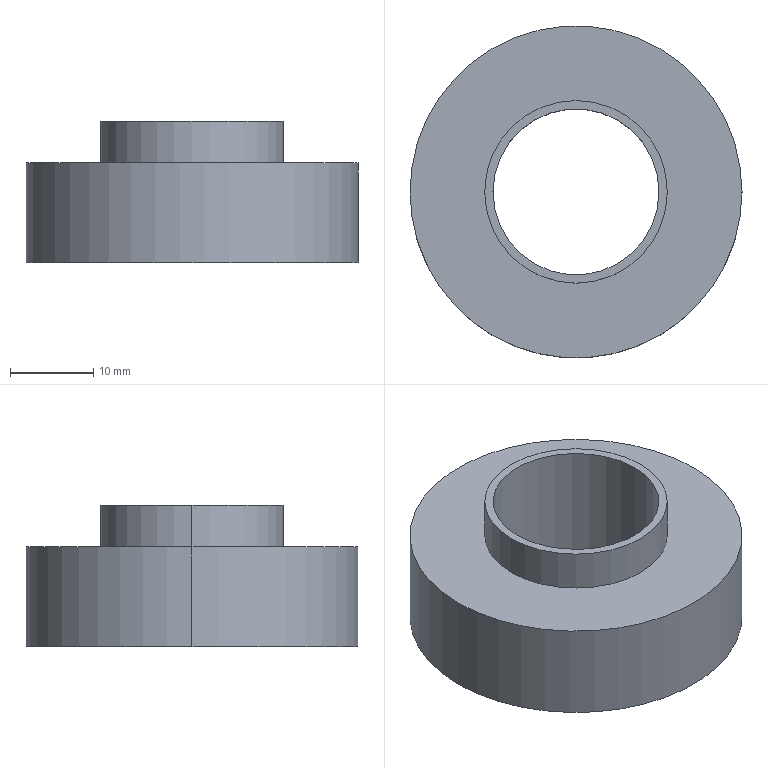Part | SolidWorks | features Extrusion 1, ICE 1 | 1 solid | 9 faces | box 40 x 40 x 17 mm | volume 11640 mm3 | cylinder 6 | plane 3 | commonest cylinder face diameters 20 x2 22 x2 40 x2
STEP:
#1=CARTESIAN_POINT('',(11.,0.,17.));
#2=VERTEX_POINT('',#1);
#3=CARTESIAN_POINT('',(-11.,0.,17.));
#4=VERTEX_POINT('',#3);
#5=CARTESIAN_POINT('',(0.,0.,17.));
#6=DIRECTION('',(0.,0.,1.));
#7=DIRECTION('',(1.,0.,0.));
#8=AXIS2_PLACEMENT_3D('',#5,#6,#7);
#9=CIRCLE('',#8,11.);
#10=EDGE_CURVE('',#2,#4,#9,.T.);
#11=ORIENTED_EDGE('',*,*,#10,.F.);
#12=CARTESIAN_POINT('',(11.,0.,12.));
#13=VERTEX_POINT('',#12);
#14=CARTESIAN_POINT('',(11.,0.,17.));
#15=DIRECTION('',(0.,0.,-1.));
#16=VECTOR('',#15,1000.);
#17=LINE('',#14,#16);
#18=EDGE_CURVE('',#2,#13,#17,.T.);
#19=ORIENTED_EDGE('',*,*,#18,.T.);
#20=CARTESIAN_POINT('',(-11.,0.,12.));
#21=VERTEX_POINT('',#20);
#22=CARTESIAN_POINT('',(0.,0.,12.));
#23=DIRECTION('',(0.,0.,1.));
#24=DIRECTION('',(1.,0.,0.));
#25=AXIS2_PLACEMENT_3D('',#22,#23,#24);
#26=CIRCLE('',#25,11.);
#27=EDGE_CURVE('',#13,#21,#26,.T.);
#28=ORIENTED_EDGE('',*,*,#27,.T.);
#29=CARTESIAN_POINT('',(-11.,0.,17.));
#30=DIRECTION('',(0.,0.,-1.));
#31=VECTOR('',#30,1000.);
#32=LINE('',#29,#31);
#33=EDGE_CURVE('',#4,#21,#32,.T.);
#34=ORIENTED_EDGE('',*,*,#33,.F.);
#35=EDGE_LOOP('',(#11,#19,#28,#34));
#36=FACE_OUTER_BOUND('',#35,.T.);
#37=CARTESIAN_POINT('',(0.,0.,17.));
#38=DIRECTION('',(0.,0.,-1.));
#39=DIRECTION('',(-1.,0.,0.));
#40=AXIS2_PLACEMENT_3D('',#37,#38,#39);
#41=CYLINDRICAL_SURFACE('',#40,11.);
#42=ADVANCED_FACE('',(#36),#41,.T.);
#43=CARTESIAN_POINT('',(-10.,0.,17.));
#44=VERTEX_POINT('',#43);
#45=CARTESIAN_POINT('',(10.,0.,17.));
#46=VERTEX_POINT('',#45);
#47=CARTESIAN_POINT('',(0.,0.,17.));
#48=DIRECTION('',(0.,0.,1.));
#49=DIRECTION('',(1.,0.,0.));
#50=AXIS2_PLACEMENT_3D('',#47,#48,#49);
#51=CIRCLE('',#50,10.);
#52=EDGE_CURVE('',#44,#46,#51,.T.);
#53=ORIENTED_EDGE('',*,*,#52,.T.);
#54=CARTESIAN_POINT('',(10.,0.,0.));
#55=VERTEX_POINT('',#54);
#56=CARTESIAN_POINT('',(10.,0.,12.));
#57=DIRECTION('',(0.,0.,-1.));
#58=VECTOR('',#57,1000.);
#59=LINE('',#56,#58);
#60=EDGE_CURVE('',#46,#55,#59,.T.);
#61=ORIENTED_EDGE('',*,*,#60,.T.);
#62=CARTESIAN_POINT('',(-10.,0.,0.));
#63=VERTEX_POINT('',#62);
#64=CARTESIAN_POINT('',(0.,0.,0.));
#65=DIRECTION('',(0.,0.,1.));
#66=DIRECTION('',(1.,0.,0.));
#67=AXIS2_PLACEMENT_3D('',#64,#65,#66);
#68=CIRCLE('',#67,10.);
#69=EDGE_CURVE('',#63,#55,#68,.T.);
#70=ORIENTED_EDGE('',*,*,#69,.F.);
#71=CARTESIAN_POINT('',(-10.,0.,12.));
#72=DIRECTION('',(0.,0.,-1.));
#73=VECTOR('',#72,1000.);
#74=LINE('',#71,#73);
#75=EDGE_CURVE('',#44,#63,#74,.T.);
#76=ORIENTED_EDGE('',*,*,#75,.F.);
#77=EDGE_LOOP('',(#53,#61,#70,#76));
#78=FACE_OUTER_BOUND('',#77,.T.);
#79=CARTESIAN_POINT('',(0.,0.,12.));
#80=DIRECTION('',(0.,0.,-1.));
#81=DIRECTION('',(-1.,0.,0.));
#82=AXIS2_PLACEMENT_3D('',#79,#80,#81);
#83=CYLINDRICAL_SURFACE('',#82,10.);
#84=ADVANCED_FACE('',(#78),#83,.F.);
#85=CARTESIAN_POINT('',(20.,0.,12.));
#86=VERTEX_POINT('',#85);
#87=CARTESIAN_POINT('',(-20.,0.,12.));
#88=VERTEX_POINT('',#87);
#89=CARTESIAN_POINT('',(0.,0.,12.));
#90=DIRECTION('',(0.,0.,1.));
#91=DIRECTION('',(1.,0.,0.));
#92=AXIS2_PLACEMENT_3D('',#89,#90,#91);
#93=CIRCLE('',#92,20.);
#94=EDGE_CURVE('',#86,#88,#93,.T.);
#95=ORIENTED_EDGE('',*,*,#94,.F.);
#96=CARTESIAN_POINT('',(20.,0.,0.));
#97=VERTEX_POINT('',#96);
#98=CARTESIAN_POINT('',(20.,0.,12.));
#99=DIRECTION('',(0.,0.,-1.));
#100=VECTOR('',#99,1000.);
#101=LINE('',#98,#100);
#102=EDGE_CURVE('',#86,#97,#101,.T.);
#103=ORIENTED_EDGE('',*,*,#102,.T.);
#104=CARTESIAN_POINT('',(-20.,0.,0.));
#105=VERTEX_POINT('',#104);
#106=CARTESIAN_POINT('',(0.,0.,0.));
#107=DIRECTION('',(0.,0.,1.));
#108=DIRECTION('',(1.,0.,0.));
#109=AXIS2_PLACEMENT_3D('',#106,#107,#108);
#110=CIRCLE('',#109,20.);
#111=EDGE_CURVE('',#97,#105,#110,.T.);
#112=ORIENTED_EDGE('',*,*,#111,.T.);
#113=CARTESIAN_POINT('',(-20.,0.,12.));
#114=DIRECTION('',(0.,0.,-1.));
#115=VECTOR('',#114,1000.);
#116=LINE('',#113,#115);
#117=EDGE_CURVE('',#88,#105,#116,.T.);
#118=ORIENTED_EDGE('',*,*,#117,.F.);
#119=EDGE_LOOP('',(#95,#103,#112,#118));
#120=FACE_OUTER_BOUND('',#119,.T.);
#121=CARTESIAN_POINT('',(0.,0.,12.));
#122=DIRECTION('',(0.,0.,-1.));
#123=DIRECTION('',(-1.,0.,0.));
#124=AXIS2_PLACEMENT_3D('',#121,#122,#123);
#125=CYLINDRICAL_SURFACE('',#124,20.);
#126=ADVANCED_FACE('',(#120),#125,.T.);
#127=CARTESIAN_POINT('',(0.,0.,12.));
#128=DIRECTION('',(0.,0.,1.));
#129=DIRECTION('',(1.,0.,0.));
#130=AXIS2_PLACEMENT_3D('',#127,#128,#129);
#131=CIRCLE('',#130,20.);
#132=EDGE_CURVE('',#88,#86,#131,.T.);
#133=ORIENTED_EDGE('',*,*,#132,.T.);
#134=ORIENTED_EDGE('',*,*,#94,.T.);
#135=EDGE_LOOP('',(#133,#134));
#136=FACE_OUTER_BOUND('',#135,.T.);
#137=CARTESIAN_POINT('',(0.,0.,12.));
#138=DIRECTION('',(0.,0.,1.));
#139=DIRECTION('',(1.,0.,0.));
#140=AXIS2_PLACEMENT_3D('',#137,#138,#139);
#141=CIRCLE('',#140,11.);
#142=EDGE_CURVE('',#21,#13,#141,.T.);
#143=ORIENTED_EDGE('',*,*,#142,.F.);
#144=ORIENTED_EDGE('',*,*,#27,.F.);
#145=EDGE_LOOP('',(#143,#144));
#146=FACE_BOUND('',#145,.T.);
#147=CARTESIAN_POINT('',(0.,0.,12.));
#148=DIRECTION('',(0.,0.,1.));
#149=DIRECTION('',(1.,0.,0.));
#150=AXIS2_PLACEMENT_3D('',#147,#148,#149);
#151=PLANE('',#150);
#152=ADVANCED_FACE('',(#136,#146),#151,.T.);
#153=CARTESIAN_POINT('',(0.,0.,0.));
#154=DIRECTION('',(0.,0.,1.));
#155=DIRECTION('',(1.,0.,0.));
#156=AXIS2_PLACEMENT_3D('',#153,#154,#155);
#157=CIRCLE('',#156,20.);
#158=EDGE_CURVE('',#105,#97,#157,.T.);
#159=ORIENTED_EDGE('',*,*,#158,.F.);
#160=ORIENTED_EDGE('',*,*,#111,.F.);
#161=EDGE_LOOP('',(#159,#160));
#162=FACE_OUTER_BOUND('',#161,.T.);
#163=ORIENTED_EDGE('',*,*,#69,.T.);
#164=CARTESIAN_POINT('',(0.,0.,0.));
#165=DIRECTION('',(0.,0.,1.));
#166=DIRECTION('',(1.,0.,0.));
#167=AXIS2_PLACEMENT_3D('',#164,#165,#166);
#168=CIRCLE('',#167,10.);
#169=EDGE_CURVE('',#55,#63,#168,.T.);
#170=ORIENTED_EDGE('',*,*,#169,.T.);
#171=EDGE_LOOP('',(#163,#170));
#172=FACE_BOUND('',#171,.T.);
#173=CARTESIAN_POINT('',(0.,0.,0.));
#174=DIRECTION('',(0.,0.,1.));
#175=DIRECTION('',(1.,0.,0.));
#176=AXIS2_PLACEMENT_3D('',#173,#174,#175);
#177=PLANE('',#176);
#178=ADVANCED_FACE('',(#162,#172),#177,.F.);
#179=ORIENTED_EDGE('',*,*,#102,.F.);
#180=ORIENTED_EDGE('',*,*,#132,.F.);
#181=ORIENTED_EDGE('',*,*,#117,.T.);
#182=ORIENTED_EDGE('',*,*,#158,.T.);
#183=EDGE_LOOP('',(#179,#180,#181,#182));
#184=FACE_OUTER_BOUND('',#183,.T.);
#185=CARTESIAN_POINT('',(0.,0.,12.));
#186=DIRECTION('',(0.,0.,-1.));
#187=DIRECTION('',(-1.,0.,0.));
#188=AXIS2_PLACEMENT_3D('',#185,#186,#187);
#189=CYLINDRICAL_SURFACE('',#188,20.);
#190=ADVANCED_FACE('',(#184),#189,.T.);
#191=ORIENTED_EDGE('',*,*,#60,.F.);
#192=CARTESIAN_POINT('',(0.,0.,17.));
#193=DIRECTION('',(0.,0.,1.));
#194=DIRECTION('',(1.,0.,0.));
#195=AXIS2_PLACEMENT_3D('',#192,#193,#194);
#196=CIRCLE('',#195,10.);
#197=EDGE_CURVE('',#46,#44,#196,.T.);
#198=ORIENTED_EDGE('',*,*,#197,.T.);
#199=ORIENTED_EDGE('',*,*,#75,.T.);
#200=ORIENTED_EDGE('',*,*,#169,.F.);
#201=EDGE_LOOP('',(#191,#198,#199,#200));
#202=FACE_OUTER_BOUND('',#201,.T.);
#203=CARTESIAN_POINT('',(0.,0.,12.));
#204=DIRECTION('',(0.,0.,-1.));
#205=DIRECTION('',(-1.,0.,0.));
#206=AXIS2_PLACEMENT_3D('',#203,#204,#205);
#207=CYLINDRICAL_SURFACE('',#206,10.);
#208=ADVANCED_FACE('',(#202),#207,.F.);
#209=CARTESIAN_POINT('',(0.,0.,17.));
#210=DIRECTION('',(0.,0.,1.));
#211=DIRECTION('',(1.,0.,0.));
#212=AXIS2_PLACEMENT_3D('',#209,#210,#211);
#213=CIRCLE('',#212,11.);
#214=EDGE_CURVE('',#4,#2,#213,.T.);
#215=ORIENTED_EDGE('',*,*,#214,.T.);
#216=ORIENTED_EDGE('',*,*,#10,.T.);
#217=EDGE_LOOP('',(#215,#216));
#218=FACE_OUTER_BOUND('',#217,.T.);
#219=ORIENTED_EDGE('',*,*,#52,.F.);
#220=ORIENTED_EDGE('',*,*,#197,.F.);
#221=EDGE_LOOP('',(#219,#220));
#222=FACE_BOUND('',#221,.T.);
#223=CARTESIAN_POINT('',(0.,0.,17.));
#224=DIRECTION('',(0.,0.,1.));
#225=DIRECTION('',(1.,0.,0.));
#226=AXIS2_PLACEMENT_3D('',#223,#224,#225);
#227=PLANE('',#226);
#228=ADVANCED_FACE('',(#218,#222),#227,.T.);
#229=ORIENTED_EDGE('',*,*,#18,.F.);
#230=ORIENTED_EDGE('',*,*,#214,.F.);
#231=ORIENTED_EDGE('',*,*,#33,.T.);
#232=ORIENTED_EDGE('',*,*,#142,.T.);
#233=EDGE_LOOP('',(#229,#230,#231,#232));
#234=FACE_OUTER_BOUND('',#233,.T.);
#235=CARTESIAN_POINT('',(0.,0.,17.));
#236=DIRECTION('',(0.,0.,-1.));
#237=DIRECTION('',(-1.,0.,0.));
#238=AXIS2_PLACEMENT_3D('',#235,#236,#237);
#239=CYLINDRICAL_SURFACE('',#238,11.);
#240=ADVANCED_FACE('',(#234),#239,.T.);
#241=CLOSED_SHELL('',(#42,#84,#126,#152,#178,#190,#208,#228,#240));
#242=MANIFOLD_SOLID_BREP('',#241);
#243=CARTESIAN_POINT('',(0.,0.,0.));
#244=DIRECTION('',(0.,0.,1.));
#245=DIRECTION('',(1.,0.,0.));
#246=AXIS2_PLACEMENT_3D('',#243,#244,#245);
#247=(LENGTH_UNIT()NAMED_UNIT(*)SI_UNIT(.MILLI.,.METRE.));
#248=UNCERTAINTY_MEASURE_WITH_UNIT(LENGTH_MEASURE(0.00001),#247,'','');
#249=(NAMED_UNIT(*)PLANE_ANGLE_UNIT()SI_UNIT($,.RADIAN.));
#250=(NAMED_UNIT(*)SI_UNIT($,.STERADIAN.)SOLID_ANGLE_UNIT());
#251=(GEOMETRIC_REPRESENTATION_CONTEXT(3)GLOBAL_UNCERTAINTY_ASSIGNED_CONTEXT((#248))GLOBAL_UNIT_ASSIGNED_CONTEXT((#247,#249,#250))REPRESENTATION_CONTEXT('',''));
#252=ADVANCED_BREP_SHAPE_REPRESENTATION('',(#242,#246),#251);